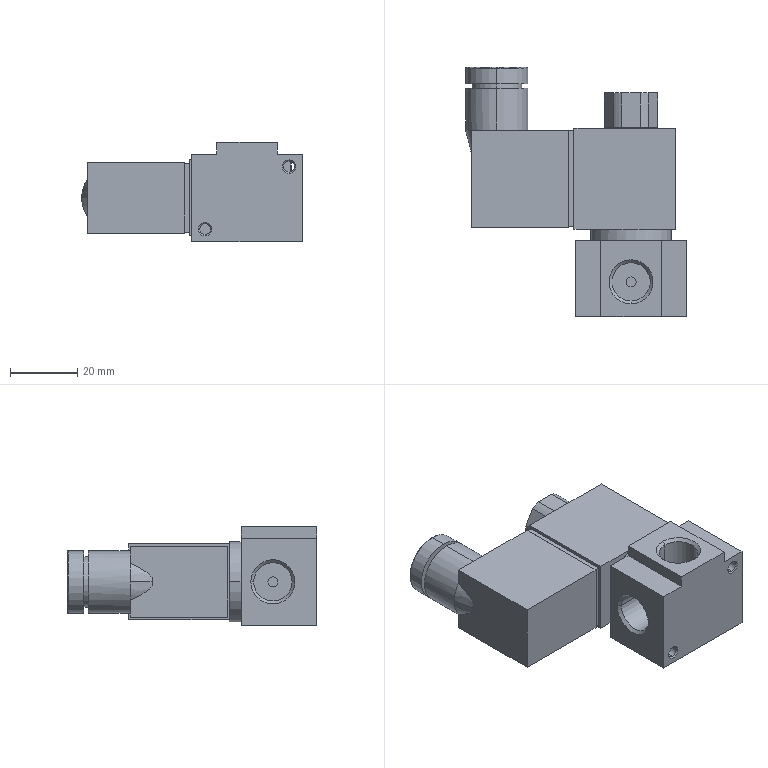Part | 1 solid | 110 faces | box 65.8 x 74.2 x 29.5 mm | volume 62036 mm3 | plane 52 | cylinder 44 | cone 12 | spline 2 | commonest cylinder face diameters 16 x7 3 x6 11.445 x6 3.242 x4 3.3 x4 6 x4